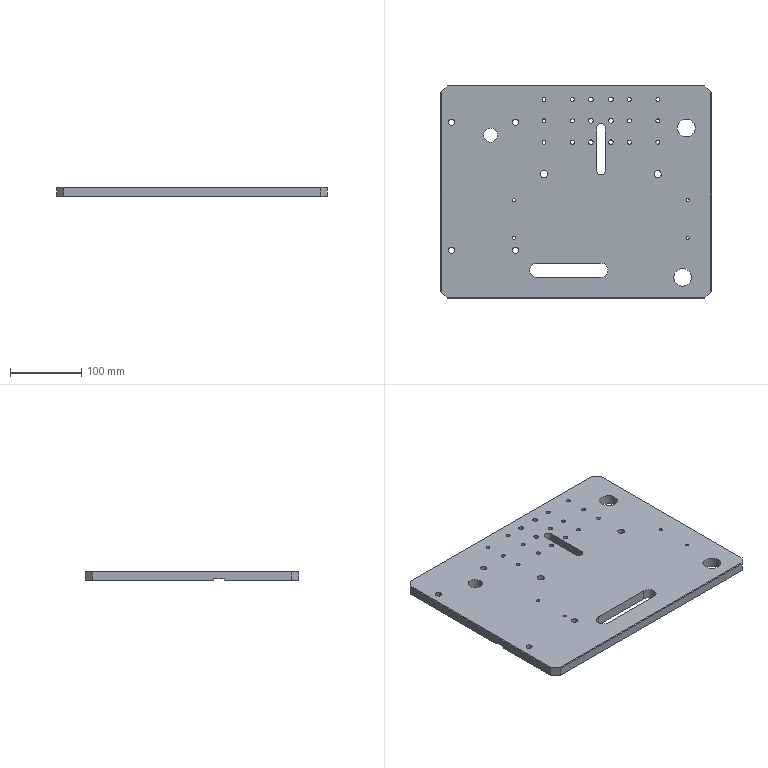Part | STEP file | Base plate | 1 solid | 163 faces | box 380 x 300 x 14 mm | volume 1501141 mm3 | cylinder 101 | cone 34 | plane 28 | commonest cylinder face diameters 3.3 x24 5.5 x24 6.5 x12 2.5 x10 4.2 x8 8.5 x8